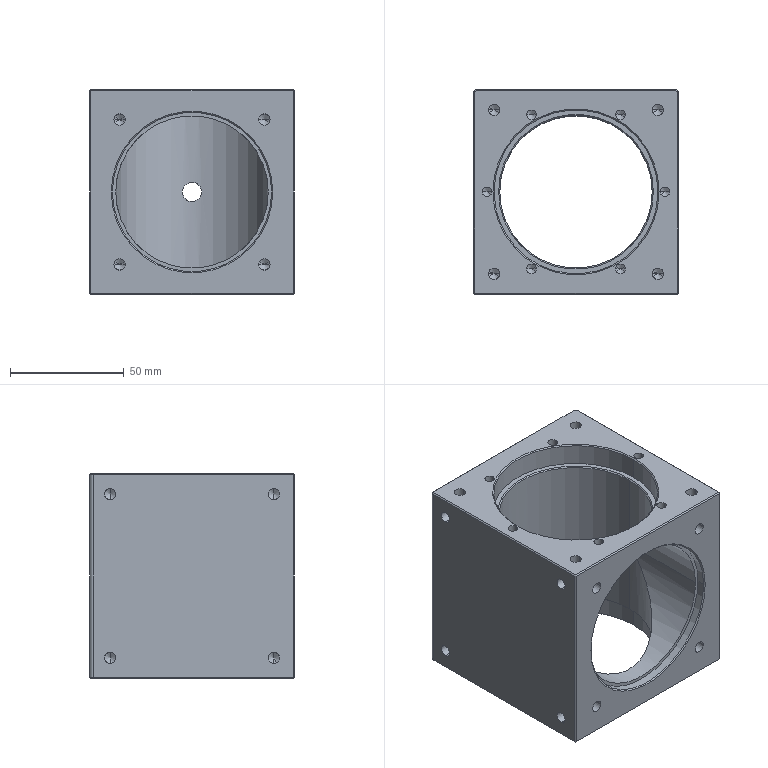Part | 1 solid | 236 faces | box 90 x 90 x 90 mm | volume 330525 mm3 | cylinder 127 | cone 86 | plane 23 | commonest cylinder face diameters 5 x88 4.2 x24 67 x5 72 x4 3 x2 8.5 x2